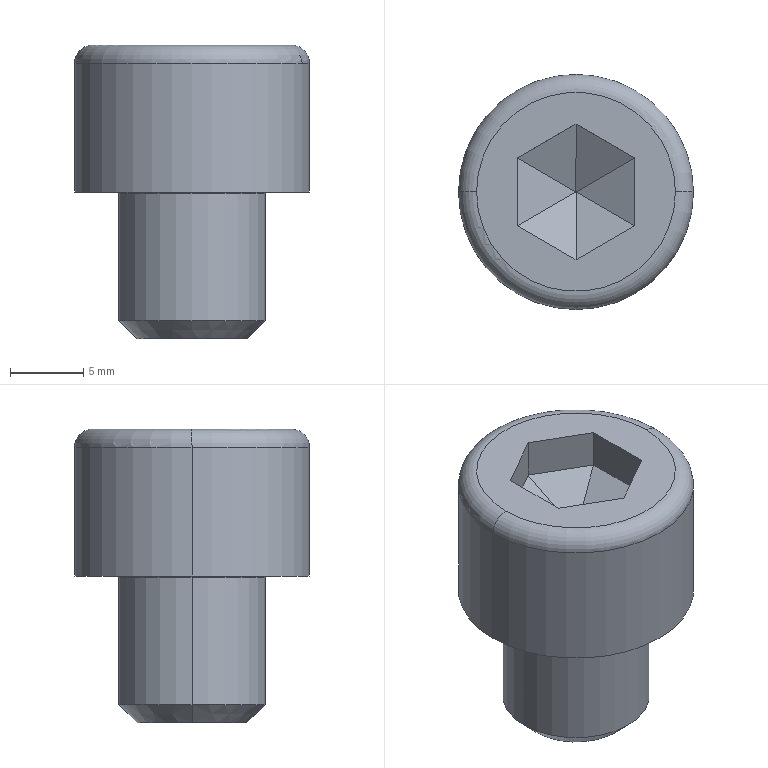Part | SolidWorks | features Chamfer 2, Fillet 2, ICE 2, Extrusion 1, RefAxis 1 | 1 solid | 26 faces | box 16 x 16 x 20 mm | volume 2566 mm3 | plane 16 | torus 4 | cylinder 4 | cone 2 | commonest cylinder face diameters 10 x2 16 x2
STEP:
#1=CARTESIAN_POINT('',(-5.1,0.,0.));
#2=VERTEX_POINT('',#1);
#3=CARTESIAN_POINT('',(5.1,0.,0.));
#4=VERTEX_POINT('',#3);
#5=CARTESIAN_POINT('',(0.,0.,0.));
#6=DIRECTION('',(0.,0.,1.));
#7=DIRECTION('',(1.,0.,0.));
#8=AXIS2_PLACEMENT_3D('',#5,#6,#7);
#9=CIRCLE('',#8,5.1);
#10=EDGE_CURVE('',#2,#4,#9,.T.);
#11=ORIENTED_EDGE('',*,*,#10,.F.);
#12=CARTESIAN_POINT('',(-5.,0.,-0.1));
#13=VERTEX_POINT('',#12);
#14=CARTESIAN_POINT('',(-5.1,0.,-0.1));
#15=DIRECTION('',(0.,1.,0.));
#16=DIRECTION('',(-1.,0.,0.));
#17=AXIS2_PLACEMENT_3D('',#14,#15,#16);
#18=CIRCLE('',#17,0.1);
#19=EDGE_CURVE('',#2,#13,#18,.T.);
#20=ORIENTED_EDGE('',*,*,#19,.T.);
#21=CARTESIAN_POINT('',(5.,0.,-0.1));
#22=VERTEX_POINT('',#21);
#23=CARTESIAN_POINT('',(0.,0.,-0.1));
#24=DIRECTION('',(0.,0.,-1.));
#25=DIRECTION('',(1.,0.,0.));
#26=AXIS2_PLACEMENT_3D('',#23,#24,#25);
#27=CIRCLE('',#26,5.);
#28=EDGE_CURVE('',#22,#13,#27,.T.);
#29=ORIENTED_EDGE('',*,*,#28,.F.);
#30=CARTESIAN_POINT('',(5.1,0.,-0.1));
#31=DIRECTION('',(0.,-1.,0.));
#32=DIRECTION('',(0.,0.,-1.));
#33=AXIS2_PLACEMENT_3D('',#30,#31,#32);
#34=CIRCLE('',#33,0.1);
#35=EDGE_CURVE('',#4,#22,#34,.T.);
#36=ORIENTED_EDGE('',*,*,#35,.F.);
#37=EDGE_LOOP('',(#11,#20,#29,#36));
#38=FACE_OUTER_BOUND('',#37,.T.);
#39=CARTESIAN_POINT('',(0.,0.,-0.1));
#40=DIRECTION('',(0.,0.,1.));
#41=DIRECTION('',(1.,0.,0.));
#42=AXIS2_PLACEMENT_3D('',#39,#40,#41);
#43=TOROIDAL_SURFACE('',#42,5.1,0.1);
#44=ADVANCED_FACE('',(#38),#43,.F.);
#45=CARTESIAN_POINT('',(-8.,0.,8.769));
#46=VERTEX_POINT('',#45);
#47=CARTESIAN_POINT('',(8.,0.,8.769));
#48=VERTEX_POINT('',#47);
#49=CARTESIAN_POINT('',(0.,0.,8.769));
#50=DIRECTION('',(0.,0.,-1.));
#51=DIRECTION('',(1.,0.,0.));
#52=AXIS2_PLACEMENT_3D('',#49,#50,#51);
#53=CIRCLE('',#52,8.);
#54=EDGE_CURVE('',#46,#48,#53,.T.);
#55=ORIENTED_EDGE('',*,*,#54,.F.);
#56=CARTESIAN_POINT('',(-6.769,0.,10.));
#57=VERTEX_POINT('',#56);
#58=CARTESIAN_POINT('',(-6.769,0.,8.769));
#59=DIRECTION('',(0.,1.,0.));
#60=DIRECTION('',(-1.,0.,0.));
#61=AXIS2_PLACEMENT_3D('',#58,#59,#60);
#62=CIRCLE('',#61,1.231);
#63=EDGE_CURVE('',#46,#57,#62,.T.);
#64=ORIENTED_EDGE('',*,*,#63,.T.);
#65=CARTESIAN_POINT('',(6.769,0.,10.));
#66=VERTEX_POINT('',#65);
#67=CARTESIAN_POINT('',(0.,0.,10.));
#68=DIRECTION('',(0.,0.,1.));
#69=DIRECTION('',(1.,0.,0.));
#70=AXIS2_PLACEMENT_3D('',#67,#68,#69);
#71=CIRCLE('',#70,6.769);
#72=EDGE_CURVE('',#66,#57,#71,.T.);
#73=ORIENTED_EDGE('',*,*,#72,.F.);
#74=CARTESIAN_POINT('',(6.769,0.,8.769));
#75=DIRECTION('',(0.,-1.,0.));
#76=DIRECTION('',(0.,0.,-1.));
#77=AXIS2_PLACEMENT_3D('',#74,#75,#76);
#78=CIRCLE('',#77,1.231);
#79=EDGE_CURVE('',#48,#66,#78,.T.);
#80=ORIENTED_EDGE('',*,*,#79,.F.);
#81=EDGE_LOOP('',(#55,#64,#73,#80));
#82=FACE_OUTER_BOUND('',#81,.T.);
#83=CARTESIAN_POINT('',(0.,0.,8.769));
#84=DIRECTION('',(0.,0.,1.));
#85=DIRECTION('',(1.,0.,0.));
#86=AXIS2_PLACEMENT_3D('',#83,#84,#85);
#87=TOROIDAL_SURFACE('',#86,6.769,1.231);
#88=ADVANCED_FACE('',(#82),#87,.T.);
#89=CARTESIAN_POINT('',(-3.75,0.,-10.));
#90=VERTEX_POINT('',#89);
#91=CARTESIAN_POINT('',(3.75,0.,-10.));
#92=VERTEX_POINT('',#91);
#93=CARTESIAN_POINT('',(0.,0.,-10.));
#94=DIRECTION('',(0.,0.,-1.));
#95=DIRECTION('',(-1.,0.,0.));
#96=AXIS2_PLACEMENT_3D('',#93,#94,#95);
#97=CIRCLE('',#96,3.75);
#98=EDGE_CURVE('',#90,#92,#97,.T.);
#99=ORIENTED_EDGE('',*,*,#98,.F.);
#100=CARTESIAN_POINT('',(-5.,0.,-8.75));
#101=VERTEX_POINT('',#100);
#102=CARTESIAN_POINT('',(-3.75,0.,-10.));
#103=DIRECTION('',(-0.7071,0.,0.7071));
#104=VECTOR('',#103,1000.);
#105=LINE('',#102,#104);
#106=EDGE_CURVE('',#90,#101,#105,.T.);
#107=ORIENTED_EDGE('',*,*,#106,.T.);
#108=CARTESIAN_POINT('',(5.,0.,-8.75));
#109=VERTEX_POINT('',#108);
#110=CARTESIAN_POINT('',(0.,0.,-8.75));
#111=DIRECTION('',(0.,0.,1.));
#112=DIRECTION('',(-1.,0.,0.));
#113=AXIS2_PLACEMENT_3D('',#110,#111,#112);
#114=CIRCLE('',#113,5.);
#115=EDGE_CURVE('',#109,#101,#114,.T.);
#116=ORIENTED_EDGE('',*,*,#115,.F.);
#117=CARTESIAN_POINT('',(3.75,0.,-10.));
#118=DIRECTION('',(0.7071,0.,0.7071));
#119=VECTOR('',#118,1000.);
#120=LINE('',#117,#119);
#121=EDGE_CURVE('',#92,#109,#120,.T.);
#122=ORIENTED_EDGE('',*,*,#121,.F.);
#123=EDGE_LOOP('',(#99,#107,#116,#122));
#124=FACE_OUTER_BOUND('',#123,.T.);
#125=CARTESIAN_POINT('',(0.,0.,-10.));
#126=DIRECTION('',(0.,0.,1.));
#127=DIRECTION('',(1.,0.,0.));
#128=AXIS2_PLACEMENT_3D('',#125,#126,#127);
#129=CONICAL_SURFACE('',#128,3.75,0.7854);
#130=ADVANCED_FACE('',(#124),#129,.T.);
#131=ORIENTED_EDGE('',*,*,#115,.T.);
#132=CARTESIAN_POINT('',(-5.,0.,-10.));
#133=DIRECTION('',(0.,0.,1.));
#134=VECTOR('',#133,1000.);
#135=LINE('',#132,#134);
#136=EDGE_CURVE('',#101,#13,#135,.T.);
#137=ORIENTED_EDGE('',*,*,#136,.T.);
#138=CARTESIAN_POINT('',(0.,0.,-0.1));
#139=DIRECTION('',(0.,0.,-1.));
#140=DIRECTION('',(1.,0.,0.));
#141=AXIS2_PLACEMENT_3D('',#138,#139,#140);
#142=CIRCLE('',#141,5.);
#143=EDGE_CURVE('',#13,#22,#142,.T.);
#144=ORIENTED_EDGE('',*,*,#143,.T.);
#145=CARTESIAN_POINT('',(5.,0.,-10.));
#146=DIRECTION('',(0.,0.,1.));
#147=VECTOR('',#146,1000.);
#148=LINE('',#145,#147);
#149=EDGE_CURVE('',#109,#22,#148,.T.);
#150=ORIENTED_EDGE('',*,*,#149,.F.);
#151=EDGE_LOOP('',(#131,#137,#144,#150));
#152=FACE_OUTER_BOUND('',#151,.T.);
#153=CARTESIAN_POINT('',(0.,0.,-10.));
#154=DIRECTION('',(0.,0.,1.));
#155=DIRECTION('',(1.,0.,0.));
#156=AXIS2_PLACEMENT_3D('',#153,#154,#155);
#157=CYLINDRICAL_SURFACE('',#156,5.);
#158=ADVANCED_FACE('',(#152),#157,.T.);
#159=ORIENTED_EDGE('',*,*,#54,.T.);
#160=CARTESIAN_POINT('',(8.,0.,0.));
#161=VERTEX_POINT('',#160);
#162=CARTESIAN_POINT('',(8.,0.,10.));
#163=DIRECTION('',(0.,0.,-1.));
#164=VECTOR('',#163,1000.);
#165=LINE('',#162,#164);
#166=EDGE_CURVE('',#48,#161,#165,.T.);
#167=ORIENTED_EDGE('',*,*,#166,.T.);
#168=CARTESIAN_POINT('',(-8.,0.,0.));
#169=VERTEX_POINT('',#168);
#170=CARTESIAN_POINT('',(0.,0.,0.));
#171=DIRECTION('',(0.,0.,1.));
#172=DIRECTION('',(1.,0.,0.));
#173=AXIS2_PLACEMENT_3D('',#170,#171,#172);
#174=CIRCLE('',#173,8.);
#175=EDGE_CURVE('',#161,#169,#174,.T.);
#176=ORIENTED_EDGE('',*,*,#175,.T.);
#177=CARTESIAN_POINT('',(-8.,0.,10.));
#178=DIRECTION('',(0.,0.,-1.));
#179=VECTOR('',#178,1000.);
#180=LINE('',#177,#179);
#181=EDGE_CURVE('',#46,#169,#180,.T.);
#182=ORIENTED_EDGE('',*,*,#181,.F.);
#183=EDGE_LOOP('',(#159,#167,#176,#182));
#184=FACE_OUTER_BOUND('',#183,.T.);
#185=CARTESIAN_POINT('',(0.,0.,10.));
#186=DIRECTION('',(0.,0.,-1.));
#187=DIRECTION('',(-1.,0.,0.));
#188=AXIS2_PLACEMENT_3D('',#185,#186,#187);
#189=CYLINDRICAL_SURFACE('',#188,8.);
#190=ADVANCED_FACE('',(#184),#189,.T.);
#191=CARTESIAN_POINT('',(0.,0.,0.));
#192=DIRECTION('',(0.,0.,1.));
#193=DIRECTION('',(1.,0.,0.));
#194=AXIS2_PLACEMENT_3D('',#191,#192,#193);
#195=CIRCLE('',#194,5.1);
#196=EDGE_CURVE('',#4,#2,#195,.T.);
#197=ORIENTED_EDGE('',*,*,#196,.T.);
#198=ORIENTED_EDGE('',*,*,#10,.T.);
#199=EDGE_LOOP('',(#197,#198));
#200=FACE_BOUND('',#199,.T.);
#201=CARTESIAN_POINT('',(0.,0.,0.));
#202=DIRECTION('',(0.,0.,1.));
#203=DIRECTION('',(1.,0.,0.));
#204=AXIS2_PLACEMENT_3D('',#201,#202,#203);
#205=CIRCLE('',#204,8.);
#206=EDGE_CURVE('',#169,#161,#205,.T.);
#207=ORIENTED_EDGE('',*,*,#206,.F.);
#208=ORIENTED_EDGE('',*,*,#175,.F.);
#209=EDGE_LOOP('',(#207,#208));
#210=FACE_OUTER_BOUND('',#209,.T.);
#211=CARTESIAN_POINT('',(0.,0.,0.));
#212=DIRECTION('',(0.,0.,1.));
#213=DIRECTION('',(1.,0.,0.));
#214=AXIS2_PLACEMENT_3D('',#211,#212,#213);
#215=PLANE('',#214);
#216=ADVANCED_FACE('',(#200,#210),#215,.F.);
#217=ORIENTED_EDGE('',*,*,#166,.F.);
#218=CARTESIAN_POINT('',(0.,0.,8.769));
#219=DIRECTION('',(0.,0.,-1.));
#220=DIRECTION('',(1.,0.,0.));
#221=AXIS2_PLACEMENT_3D('',#218,#219,#220);
#222=CIRCLE('',#221,8.);
#223=EDGE_CURVE('',#48,#46,#222,.T.);
#224=ORIENTED_EDGE('',*,*,#223,.T.);
#225=ORIENTED_EDGE('',*,*,#181,.T.);
#226=ORIENTED_EDGE('',*,*,#206,.T.);
#227=EDGE_LOOP('',(#217,#224,#225,#226));
#228=FACE_OUTER_BOUND('',#227,.T.);
#229=CARTESIAN_POINT('',(0.,0.,10.));
#230=DIRECTION('',(0.,0.,-1.));
#231=DIRECTION('',(-1.,0.,0.));
#232=AXIS2_PLACEMENT_3D('',#229,#230,#231);
#233=CYLINDRICAL_SURFACE('',#232,8.);
#234=ADVANCED_FACE('',(#228),#233,.T.);
#235=ORIENTED_EDGE('',*,*,#72,.T.);
#236=CARTESIAN_POINT('',(0.,0.,10.));
#237=DIRECTION('',(0.,0.,1.));
#238=DIRECTION('',(1.,0.,0.));
#239=AXIS2_PLACEMENT_3D('',#236,#237,#238);
#240=CIRCLE('',#239,6.769);
#241=EDGE_CURVE('',#57,#66,#240,.T.);
#242=ORIENTED_EDGE('',*,*,#241,.T.);
#243=EDGE_LOOP('',(#235,#242));
#244=FACE_OUTER_BOUND('',#243,.T.);
#245=CARTESIAN_POINT('',(4.,-2.309,10.));
#246=VERTEX_POINT('',#245);
#247=CARTESIAN_POINT('',(4.,2.309,10.));
#248=VERTEX_POINT('',#247);
#249=CARTESIAN_POINT('',(4.,-2.309,10.));
#250=DIRECTION('',(0.,1.,0.));
#251=VECTOR('',#250,1000.);
#252=LINE('',#249,#251);
#253=EDGE_CURVE('',#246,#248,#252,.T.);
#254=ORIENTED_EDGE('',*,*,#253,.F.);
#255=CARTESIAN_POINT('',(0.,-4.619,10.));
#256=VERTEX_POINT('',#255);
#257=CARTESIAN_POINT('',(0.,-4.619,10.));
#258=DIRECTION('',(0.866,0.5,0.));
#259=VECTOR('',#258,1000.);
#260=LINE('',#257,#259);
#261=EDGE_CURVE('',#256,#246,#260,.T.);
#262=ORIENTED_EDGE('',*,*,#261,.F.);
#263=CARTESIAN_POINT('',(-4.,-2.309,10.));
#264=VERTEX_POINT('',#263);
#265=CARTESIAN_POINT('',(-4.,-2.309,10.));
#266=DIRECTION('',(0.866,-0.5,0.));
#267=VECTOR('',#266,1000.);
#268=LINE('',#265,#267);
#269=EDGE_CURVE('',#264,#256,#268,.T.);
#270=ORIENTED_EDGE('',*,*,#269,.F.);
#271=CARTESIAN_POINT('',(-4.,2.309,10.));
#272=VERTEX_POINT('',#271);
#273=CARTESIAN_POINT('',(-4.,2.309,10.));
#274=DIRECTION('',(0.,-1.,0.));
#275=VECTOR('',#274,1000.);
#276=LINE('',#273,#275);
#277=EDGE_CURVE('',#272,#264,#276,.T.);
#278=ORIENTED_EDGE('',*,*,#277,.F.);
#279=CARTESIAN_POINT('',(0.,4.619,10.));
#280=VERTEX_POINT('',#279);
#281=CARTESIAN_POINT('',(0.,4.619,10.));
#282=DIRECTION('',(-0.866,-0.5,0.));
#283=VECTOR('',#282,1000.);
#284=LINE('',#281,#283);
#285=EDGE_CURVE('',#280,#272,#284,.T.);
#286=ORIENTED_EDGE('',*,*,#285,.F.);
#287=CARTESIAN_POINT('',(4.,2.309,10.));
#288=DIRECTION('',(-0.866,0.5,0.));
#289=VECTOR('',#288,1000.);
#290=LINE('',#287,#289);
#291=EDGE_CURVE('',#248,#280,#290,.T.);
#292=ORIENTED_EDGE('',*,*,#291,.F.);
#293=EDGE_LOOP('',(#254,#262,#270,#278,#286,#292));
#294=FACE_BOUND('',#293,.T.);
#295=CARTESIAN_POINT('',(0.,0.,10.));
#296=DIRECTION('',(0.,0.,1.));
#297=DIRECTION('',(1.,0.,0.));
#298=AXIS2_PLACEMENT_3D('',#295,#296,#297);
#299=PLANE('',#298);
#300=ADVANCED_FACE('',(#244,#294),#299,.T.);
#301=CARTESIAN_POINT('',(4.,2.309,7.305));
#302=VERTEX_POINT('',#301);
#303=CARTESIAN_POINT('',(4.,2.309,5.));
#304=DIRECTION('',(0.,0.,1.));
#305=VECTOR('',#304,1000.);
#306=LINE('',#303,#305);
#307=EDGE_CURVE('',#302,#248,#306,.T.);
#308=ORIENTED_EDGE('',*,*,#307,.F.);
#309=CARTESIAN_POINT('',(4.,-2.309,7.305));
#310=VERTEX_POINT('',#309);
#311=CARTESIAN_POINT('',(4.,-2.309,7.305));
#312=DIRECTION('',(0.,-1.,0.));
#313=VECTOR('',#312,1000.);
#314=LINE('',#311,#313);
#315=EDGE_CURVE('',#302,#310,#314,.T.);
#316=ORIENTED_EDGE('',*,*,#315,.T.);
#317=CARTESIAN_POINT('',(4.,-2.309,5.));
#318=DIRECTION('',(0.,0.,1.));
#319=VECTOR('',#318,1000.);
#320=LINE('',#317,#319);
#321=EDGE_CURVE('',#310,#246,#320,.T.);
#322=ORIENTED_EDGE('',*,*,#321,.T.);
#323=ORIENTED_EDGE('',*,*,#253,.T.);
#324=EDGE_LOOP('',(#308,#316,#322,#323));
#325=FACE_OUTER_BOUND('',#324,.T.);
#326=CARTESIAN_POINT('',(4.,-2.309,5.));
#327=DIRECTION('',(1.,0.,0.));
#328=DIRECTION('',(0.,1.,0.));
#329=AXIS2_PLACEMENT_3D('',#326,#327,#328);
#330=PLANE('',#329);
#331=ADVANCED_FACE('',(#325),#330,.F.);
#332=ORIENTED_EDGE('',*,*,#321,.F.);
#333=CARTESIAN_POINT('',(0.,-4.619,7.305));
#334=VERTEX_POINT('',#333);
#335=CARTESIAN_POINT('',(0.,-4.619,7.305));
#336=DIRECTION('',(-0.866,-0.5,0.));
#337=VECTOR('',#336,1000.);
#338=LINE('',#335,#337);
#339=EDGE_CURVE('',#310,#334,#338,.T.);
#340=ORIENTED_EDGE('',*,*,#339,.T.);
#341=CARTESIAN_POINT('',(0.,-4.619,5.));
#342=DIRECTION('',(0.,0.,1.));
#343=VECTOR('',#342,1000.);
#344=LINE('',#341,#343);
#345=EDGE_CURVE('',#334,#256,#344,.T.);
#346=ORIENTED_EDGE('',*,*,#345,.T.);
#347=ORIENTED_EDGE('',*,*,#261,.T.);
#348=EDGE_LOOP('',(#332,#340,#346,#347));
#349=FACE_OUTER_BOUND('',#348,.T.);
#350=CARTESIAN_POINT('',(0.,-4.619,5.));
#351=DIRECTION('',(0.5,-0.866,0.));
#352=DIRECTION('',(0.866,0.5,0.));
#353=AXIS2_PLACEMENT_3D('',#350,#351,#352);
#354=PLANE('',#353);
#355=ADVANCED_FACE('',(#349),#354,.F.);
#356=ORIENTED_EDGE('',*,*,#345,.F.);
#357=CARTESIAN_POINT('',(-4.,-2.309,7.305));
#358=VERTEX_POINT('',#357);
#359=CARTESIAN_POINT('',(-4.,-2.309,7.305));
#360=DIRECTION('',(-0.866,0.5,0.));
#361=VECTOR('',#360,1000.);
#362=LINE('',#359,#361);
#363=EDGE_CURVE('',#334,#358,#362,.T.);
#364=ORIENTED_EDGE('',*,*,#363,.T.);
#365=CARTESIAN_POINT('',(-4.,-2.309,5.));
#366=DIRECTION('',(0.,0.,1.));
#367=VECTOR('',#366,1000.);
#368=LINE('',#365,#367);
#369=EDGE_CURVE('',#358,#264,#368,.T.);
#370=ORIENTED_EDGE('',*,*,#369,.T.);
#371=ORIENTED_EDGE('',*,*,#269,.T.);
#372=EDGE_LOOP('',(#356,#364,#370,#371));
#373=FACE_OUTER_BOUND('',#372,.T.);
#374=CARTESIAN_POINT('',(-4.,-2.309,5.));
#375=DIRECTION('',(-0.5,-0.866,0.));
#376=DIRECTION('',(0.866,-0.5,0.));
#377=AXIS2_PLACEMENT_3D('',#374,#375,#376);
#378=PLANE('',#377);
#379=ADVANCED_FACE('',(#373),#378,.F.);
#380=ORIENTED_EDGE('',*,*,#369,.F.);
#381=CARTESIAN_POINT('',(-4.,2.309,7.305));
#382=VERTEX_POINT('',#381);
#383=CARTESIAN_POINT('',(-4.,2.309,7.305));
#384=DIRECTION('',(0.,1.,0.));
#385=VECTOR('',#384,1000.);
#386=LINE('',#383,#385);
#387=EDGE_CURVE('',#358,#382,#386,.T.);
#388=ORIENTED_EDGE('',*,*,#387,.T.);
#389=CARTESIAN_POINT('',(-4.,2.309,5.));
#390=DIRECTION('',(0.,0.,1.));
#391=VECTOR('',#390,1000.);
#392=LINE('',#389,#391);
#393=EDGE_CURVE('',#382,#272,#392,.T.);
#394=ORIENTED_EDGE('',*,*,#393,.T.);
#395=ORIENTED_EDGE('',*,*,#277,.T.);
#396=EDGE_LOOP('',(#380,#388,#394,#395));
#397=FACE_OUTER_BOUND('',#396,.T.);
#398=CARTESIAN_POINT('',(-4.,2.309,5.));
#399=DIRECTION('',(-1.,0.,0.));
#400=DIRECTION('',(0.,0.,1.));
#401=AXIS2_PLACEMENT_3D('',#398,#399,#400);
#402=PLANE('',#401);
#403=ADVANCED_FACE('',(#397),#402,.F.);
#404=ORIENTED_EDGE('',*,*,#393,.F.);
#405=CARTESIAN_POINT('',(0.,4.619,7.305));
#406=VERTEX_POINT('',#405);
#407=CARTESIAN_POINT('',(0.,4.619,7.305));
#408=DIRECTION('',(0.866,0.5,0.));
#409=VECTOR('',#408,1000.);
#410=LINE('',#407,#409);
#411=EDGE_CURVE('',#382,#406,#410,.T.);
#412=ORIENTED_EDGE('',*,*,#411,.T.);
#413=CARTESIAN_POINT('',(0.,4.619,5.));
#414=DIRECTION('',(0.,0.,1.));
#415=VECTOR('',#414,1000.);
#416=LINE('',#413,#415);
#417=EDGE_CURVE('',#406,#280,#416,.T.);
#418=ORIENTED_EDGE('',*,*,#417,.T.);
#419=ORIENTED_EDGE('',*,*,#285,.T.);
#420=EDGE_LOOP('',(#404,#412,#418,#419));
#421=FACE_OUTER_BOUND('',#420,.T.);
#422=CARTESIAN_POINT('',(0.,4.619,5.));
#423=DIRECTION('',(-0.5,0.866,0.));
#424=DIRECTION('',(-0.866,-0.5,0.));
#425=AXIS2_PLACEMENT_3D('',#422,#423,#424);
#426=PLANE('',#425);
#427=ADVANCED_FACE('',(#421),#426,.F.);
#428=ORIENTED_EDGE('',*,*,#417,.F.);
#429=CARTESIAN_POINT('',(4.,2.309,7.305));
#430=DIRECTION('',(0.866,-0.5,0.));
#431=VECTOR('',#430,1000.);
#432=LINE('',#429,#431);
#433=EDGE_CURVE('',#406,#302,#432,.T.);
#434=ORIENTED_EDGE('',*,*,#433,.T.);
#435=ORIENTED_EDGE('',*,*,#307,.T.);
#436=ORIENTED_EDGE('',*,*,#291,.T.);
#437=EDGE_LOOP('',(#428,#434,#435,#436));
#438=FACE_OUTER_BOUND('',#437,.T.);
#439=CARTESIAN_POINT('',(4.,2.309,5.));
#440=DIRECTION('',(0.5,0.866,0.));
#441=DIRECTION('',(-0.866,0.5,0.));
#442=AXIS2_PLACEMENT_3D('',#439,#440,#441);
#443=PLANE('',#442);
#444=ADVANCED_FACE('',(#438),#443,.F.);
#445=CARTESIAN_POINT('',(0.,0.007851,5.));
#446=VERTEX_POINT('',#445);
#447=CARTESIAN_POINT('',(-0.006799,0.003926,5.));
#448=VERTEX_POINT('',#447);
#449=CARTESIAN_POINT('',(-0.0034,0.005888,5.));
#450=DIRECTION('',(-0.866,-0.5,0.));
#451=VECTOR('',#450,1000.);
#452=LINE('',#449,#451);
#453=EDGE_CURVE('',#446,#448,#452,.T.);
#454=ORIENTED_EDGE('',*,*,#453,.T.);
#455=CARTESIAN_POINT('',(-0.006799,-0.003926,5.));
#456=VERTEX_POINT('',#455);
#457=CARTESIAN_POINT('',(-0.006799,0.,5.));
#458=DIRECTION('',(0.,-1.,0.));
#459=VECTOR('',#458,1000.);
#460=LINE('',#457,#459);
#461=EDGE_CURVE('',#448,#456,#460,.T.);
#462=ORIENTED_EDGE('',*,*,#461,.T.);
#463=CARTESIAN_POINT('',(0.,-0.007851,5.));
#464=VERTEX_POINT('',#463);
#465=CARTESIAN_POINT('',(-0.0034,-0.005888,5.));
#466=DIRECTION('',(0.866,-0.5,0.));
#467=VECTOR('',#466,1000.);
#468=LINE('',#465,#467);
#469=EDGE_CURVE('',#456,#464,#468,.T.);
#470=ORIENTED_EDGE('',*,*,#469,.T.);
#471=CARTESIAN_POINT('',(0.006799,-0.003926,5.));
#472=VERTEX_POINT('',#471);
#473=CARTESIAN_POINT('',(0.0034,-0.005888,5.));
#474=DIRECTION('',(0.866,0.5,0.));
#475=VECTOR('',#474,1000.);
#476=LINE('',#473,#475);
#477=EDGE_CURVE('',#464,#472,#476,.T.);
#478=ORIENTED_EDGE('',*,*,#477,.T.);
#479=CARTESIAN_POINT('',(0.006799,0.003926,5.));
#480=VERTEX_POINT('',#479);
#481=CARTESIAN_POINT('',(0.006799,0.,5.));
#482=DIRECTION('',(0.,1.,0.));
#483=VECTOR('',#482,1000.);
#484=LINE('',#481,#483);
#485=EDGE_CURVE('',#472,#480,#484,.T.);
#486=ORIENTED_EDGE('',*,*,#485,.T.);
#487=CARTESIAN_POINT('',(0.0034,0.005888,5.));
#488=DIRECTION('',(-0.866,0.5,0.));
#489=VECTOR('',#488,1000.);
#490=LINE('',#487,#489);
#491=EDGE_CURVE('',#480,#446,#490,.T.);
#492=ORIENTED_EDGE('',*,*,#491,.T.);
#493=EDGE_LOOP('',(#454,#462,#470,#478,#486,#492));
#494=FACE_OUTER_BOUND('',#493,.T.);
#495=CARTESIAN_POINT('',(0.,0.,5.));
#496=DIRECTION('',(0.,0.,1.));
#497=DIRECTION('',(1.,0.,0.));
#498=AXIS2_PLACEMENT_3D('',#495,#496,#497);
#499=PLANE('',#498);
#500=ADVANCED_FACE('',(#494),#499,.T.);
#501=ORIENTED_EDGE('',*,*,#136,.F.);
#502=CARTESIAN_POINT('',(0.,0.,-8.75));
#503=DIRECTION('',(0.,0.,1.));
#504=DIRECTION('',(-1.,0.,0.));
#505=AXIS2_PLACEMENT_3D('',#502,#503,#504);
#506=CIRCLE('',#505,5.);
#507=EDGE_CURVE('',#101,#109,#506,.T.);
#508=ORIENTED_EDGE('',*,*,#507,.T.);
#509=ORIENTED_EDGE('',*,*,#149,.T.);
#510=ORIENTED_EDGE('',*,*,#28,.T.);
#511=EDGE_LOOP('',(#501,#508,#509,#510));
#512=FACE_OUTER_BOUND('',#511,.T.);
#513=CARTESIAN_POINT('',(0.,0.,-10.));
#514=DIRECTION('',(0.,0.,1.));
#515=DIRECTION('',(1.,0.,0.));
#516=AXIS2_PLACEMENT_3D('',#513,#514,#515);
#517=CYLINDRICAL_SURFACE('',#516,5.);
#518=ADVANCED_FACE('',(#512),#517,.T.);
#519=CARTESIAN_POINT('',(0.,0.,-10.));
#520=DIRECTION('',(0.,0.,-1.));
#521=DIRECTION('',(-1.,0.,0.));
#522=AXIS2_PLACEMENT_3D('',#519,#520,#521);
#523=CIRCLE('',#522,3.75);
#524=EDGE_CURVE('',#92,#90,#523,.T.);
#525=ORIENTED_EDGE('',*,*,#524,.T.);
#526=ORIENTED_EDGE('',*,*,#98,.T.);
#527=EDGE_LOOP('',(#525,#526));
#528=FACE_OUTER_BOUND('',#527,.T.);
#529=CARTESIAN_POINT('',(0.,0.,-10.));
#530=DIRECTION('',(0.,0.,-1.));
#531=DIRECTION('',(-1.,0.,0.));
#532=AXIS2_PLACEMENT_3D('',#529,#530,#531);
#533=PLANE('',#532);
#534=ADVANCED_FACE('',(#528),#533,.T.);
#535=ORIENTED_EDGE('',*,*,#106,.F.);
#536=ORIENTED_EDGE('',*,*,#524,.F.);
#537=ORIENTED_EDGE('',*,*,#121,.T.);
#538=ORIENTED_EDGE('',*,*,#507,.F.);
#539=EDGE_LOOP('',(#535,#536,#537,#538));
#540=FACE_OUTER_BOUND('',#539,.T.);
#541=CARTESIAN_POINT('',(0.,0.,-10.));
#542=DIRECTION('',(0.,0.,1.));
#543=DIRECTION('',(1.,0.,0.));
#544=AXIS2_PLACEMENT_3D('',#541,#542,#543);
#545=CONICAL_SURFACE('',#544,3.75,0.7854);
#546=ADVANCED_FACE('',(#540),#545,.T.);
#547=ORIENTED_EDGE('',*,*,#63,.F.);
#548=ORIENTED_EDGE('',*,*,#223,.F.);
#549=ORIENTED_EDGE('',*,*,#79,.T.);
#550=ORIENTED_EDGE('',*,*,#241,.F.);
#551=EDGE_LOOP('',(#547,#548,#549,#550));
#552=FACE_OUTER_BOUND('',#551,.T.);
#553=CARTESIAN_POINT('',(0.,0.,8.769));
#554=DIRECTION('',(0.,0.,1.));
#555=DIRECTION('',(1.,0.,0.));
#556=AXIS2_PLACEMENT_3D('',#553,#554,#555);
#557=TOROIDAL_SURFACE('',#556,6.769,1.231);
#558=ADVANCED_FACE('',(#552),#557,.T.);
#559=CARTESIAN_POINT('',(0.005439,-0.00314,4.999));
#560=DIRECTION('',(-0.7746,0.4472,-0.4472));
#561=VECTOR('',#560,1000.);
#562=LINE('',#559,#561);
#563=EDGE_CURVE('',#310,#472,#562,.T.);
#564=ORIENTED_EDGE('',*,*,#563,.F.);
#565=ORIENTED_EDGE('',*,*,#315,.F.);
#566=CARTESIAN_POINT('',(0.005439,0.00314,4.999));
#567=DIRECTION('',(0.7746,0.4472,0.4472));
#568=VECTOR('',#567,1000.);
#569=LINE('',#566,#568);
#570=EDGE_CURVE('',#480,#302,#569,.T.);
#571=ORIENTED_EDGE('',*,*,#570,.F.);
#572=ORIENTED_EDGE('',*,*,#485,.F.);
#573=EDGE_LOOP('',(#564,#565,#571,#572));
#574=FACE_OUTER_BOUND('',#573,.T.);
#575=CARTESIAN_POINT('',(0.006799,0.,5.));
#576=DIRECTION('',(0.5,0.,-0.866));
#577=DIRECTION('',(0.,1.,0.));
#578=AXIS2_PLACEMENT_3D('',#575,#576,#577);
#579=PLANE('',#578);
#580=ADVANCED_FACE('',(#574),#579,.F.);
#581=ORIENTED_EDGE('',*,*,#570,.T.);
#582=ORIENTED_EDGE('',*,*,#433,.F.);
#583=CARTESIAN_POINT('',(0.,0.006281,4.999));
#584=DIRECTION('',(0.,0.8944,0.4472));
#585=VECTOR('',#584,1000.);
#586=LINE('',#583,#585);
#587=EDGE_CURVE('',#446,#406,#586,.T.);
#588=ORIENTED_EDGE('',*,*,#587,.F.);
#589=ORIENTED_EDGE('',*,*,#491,.F.);
#590=EDGE_LOOP('',(#581,#582,#588,#589));
#591=FACE_OUTER_BOUND('',#590,.T.);
#592=CARTESIAN_POINT('',(0.0034,0.005888,5.));
#593=DIRECTION('',(0.25,0.433,-0.866));
#594=DIRECTION('',(-0.866,0.5,0.));
#595=AXIS2_PLACEMENT_3D('',#592,#593,#594);
#596=PLANE('',#595);
#597=ADVANCED_FACE('',(#591),#596,.F.);
#598=ORIENTED_EDGE('',*,*,#563,.T.);
#599=ORIENTED_EDGE('',*,*,#477,.F.);
#600=CARTESIAN_POINT('',(0.,-0.006281,4.999));
#601=DIRECTION('',(0.,0.8944,-0.4472));
#602=VECTOR('',#601,1000.);
#603=LINE('',#600,#602);
#604=EDGE_CURVE('',#334,#464,#603,.T.);
#605=ORIENTED_EDGE('',*,*,#604,.F.);
#606=ORIENTED_EDGE('',*,*,#339,.F.);
#607=EDGE_LOOP('',(#598,#599,#605,#606));
#608=FACE_OUTER_BOUND('',#607,.T.);
#609=CARTESIAN_POINT('',(0.0034,-0.005888,5.));
#610=DIRECTION('',(0.25,-0.433,-0.866));
#611=DIRECTION('',(0.866,0.5,0.));
#612=AXIS2_PLACEMENT_3D('',#609,#610,#611);
#613=PLANE('',#612);
#614=ADVANCED_FACE('',(#608),#613,.F.);
#615=ORIENTED_EDGE('',*,*,#587,.T.);
#616=ORIENTED_EDGE('',*,*,#411,.F.);
#617=CARTESIAN_POINT('',(-0.005439,0.00314,4.999));
#618=DIRECTION('',(-0.7746,0.4472,0.4472));
#619=VECTOR('',#618,1000.);
#620=LINE('',#617,#619);
#621=EDGE_CURVE('',#448,#382,#620,.T.);
#622=ORIENTED_EDGE('',*,*,#621,.F.);
#623=ORIENTED_EDGE('',*,*,#453,.F.);
#624=EDGE_LOOP('',(#615,#616,#622,#623));
#625=FACE_OUTER_BOUND('',#624,.T.);
#626=CARTESIAN_POINT('',(-0.0034,0.005888,5.));
#627=DIRECTION('',(-0.25,0.433,-0.866));
#628=DIRECTION('',(-0.866,-0.5,0.));
#629=AXIS2_PLACEMENT_3D('',#626,#627,#628);
#630=PLANE('',#629);
#631=ADVANCED_FACE('',(#625),#630,.F.);
#632=ORIENTED_EDGE('',*,*,#604,.T.);
#633=ORIENTED_EDGE('',*,*,#469,.F.);
#634=CARTESIAN_POINT('',(-0.005439,-0.00314,4.999));
#635=DIRECTION('',(0.7746,0.4472,-0.4472));
#636=VECTOR('',#635,1000.);
#637=LINE('',#634,#636);
#638=EDGE_CURVE('',#358,#456,#637,.T.);
#639=ORIENTED_EDGE('',*,*,#638,.F.);
#640=ORIENTED_EDGE('',*,*,#363,.F.);
#641=EDGE_LOOP('',(#632,#633,#639,#640));
#642=FACE_OUTER_BOUND('',#641,.T.);
#643=CARTESIAN_POINT('',(-0.0034,-0.005888,5.));
#644=DIRECTION('',(-0.25,-0.433,-0.866));
#645=DIRECTION('',(0.866,-0.5,0.));
#646=AXIS2_PLACEMENT_3D('',#643,#644,#645);
#647=PLANE('',#646);
#648=ADVANCED_FACE('',(#642),#647,.F.);
#649=ORIENTED_EDGE('',*,*,#621,.T.);
#650=ORIENTED_EDGE('',*,*,#387,.F.);
#651=ORIENTED_EDGE('',*,*,#638,.T.);
#652=ORIENTED_EDGE('',*,*,#461,.F.);
#653=EDGE_LOOP('',(#649,#650,#651,#652));
#654=FACE_OUTER_BOUND('',#653,.T.);
#655=CARTESIAN_POINT('',(-0.006799,0.,5.));
#656=DIRECTION('',(-0.5,0.,-0.866));
#657=DIRECTION('',(0.,-1.,0.));
#658=AXIS2_PLACEMENT_3D('',#655,#656,#657);
#659=PLANE('',#658);
#660=ADVANCED_FACE('',(#654),#659,.F.);
#661=ORIENTED_EDGE('',*,*,#19,.F.);
#662=ORIENTED_EDGE('',*,*,#196,.F.);
#663=ORIENTED_EDGE('',*,*,#35,.T.);
#664=ORIENTED_EDGE('',*,*,#143,.F.);
#665=EDGE_LOOP('',(#661,#662,#663,#664));
#666=FACE_OUTER_BOUND('',#665,.T.);
#667=CARTESIAN_POINT('',(0.,0.,-0.1));
#668=DIRECTION('',(0.,0.,1.));
#669=DIRECTION('',(1.,0.,0.));
#670=AXIS2_PLACEMENT_3D('',#667,#668,#669);
#671=TOROIDAL_SURFACE('',#670,5.1,0.1);
#672=ADVANCED_FACE('',(#666),#671,.F.);
#673=CLOSED_SHELL('',(#44,#88,#130,#158,#190,#216,#234,#300,#331,#355,#379,#403,#427,#444,#500,#518,#534,#546,#558,#580,#597,#614,#631,#648,#660,#672));
#674=MANIFOLD_SOLID_BREP('',#673);
#675=CARTESIAN_POINT('',(0.,0.,0.));
#676=DIRECTION('',(0.,0.,1.));
#677=DIRECTION('',(1.,0.,0.));
#678=AXIS2_PLACEMENT_3D('',#675,#676,#677);
#679=(LENGTH_UNIT()NAMED_UNIT(*)SI_UNIT(.MILLI.,.METRE.));
#680=UNCERTAINTY_MEASURE_WITH_UNIT(LENGTH_MEASURE(0.00001),#679,'','');
#681=(NAMED_UNIT(*)PLANE_ANGLE_UNIT()SI_UNIT($,.RADIAN.));
#682=(NAMED_UNIT(*)SI_UNIT($,.STERADIAN.)SOLID_ANGLE_UNIT());
#683=(GEOMETRIC_REPRESENTATION_CONTEXT(3)GLOBAL_UNCERTAINTY_ASSIGNED_CONTEXT((#680))GLOBAL_UNIT_ASSIGNED_CONTEXT((#679,#681,#682))REPRESENTATION_CONTEXT('',''));
#684=ADVANCED_BREP_SHAPE_REPRESENTATION('',(#674,#678),#683);